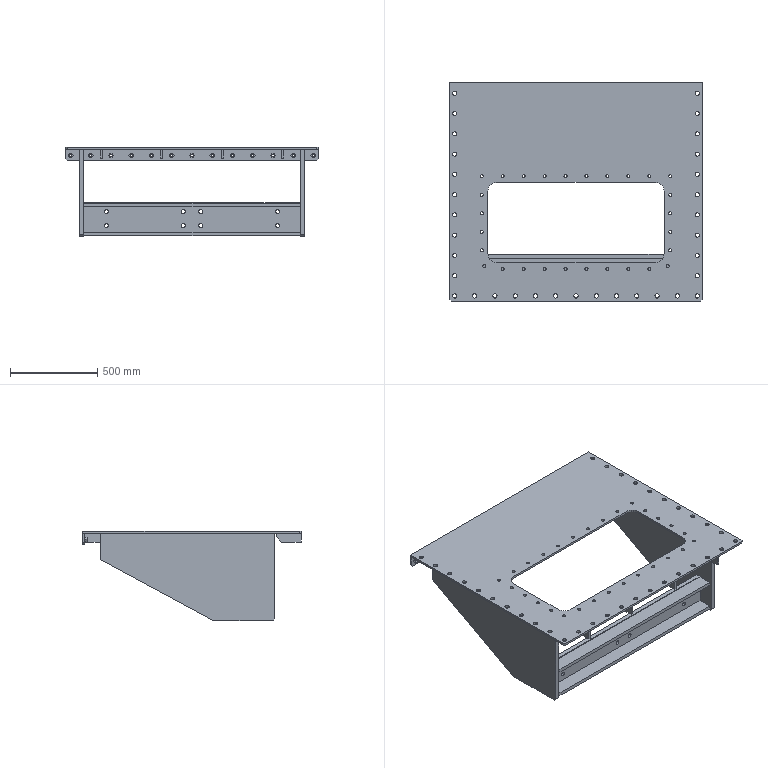Part | SolidWorks | features ICE 13, LPattern 8, Chamfer 5, HoleWzd 4, MirrorPattern 3, MirrorSolid 2, Extrusion 1, Fillet 1 | 26 solids | 406 faces | box 1448 x 1250 x 512 mm | volume 47295525 mm3 | plane 212 | cylinder 194 | commonest cylinder face diameters 24 x66 17.5 x56 14 x52 22 x16 100 x4